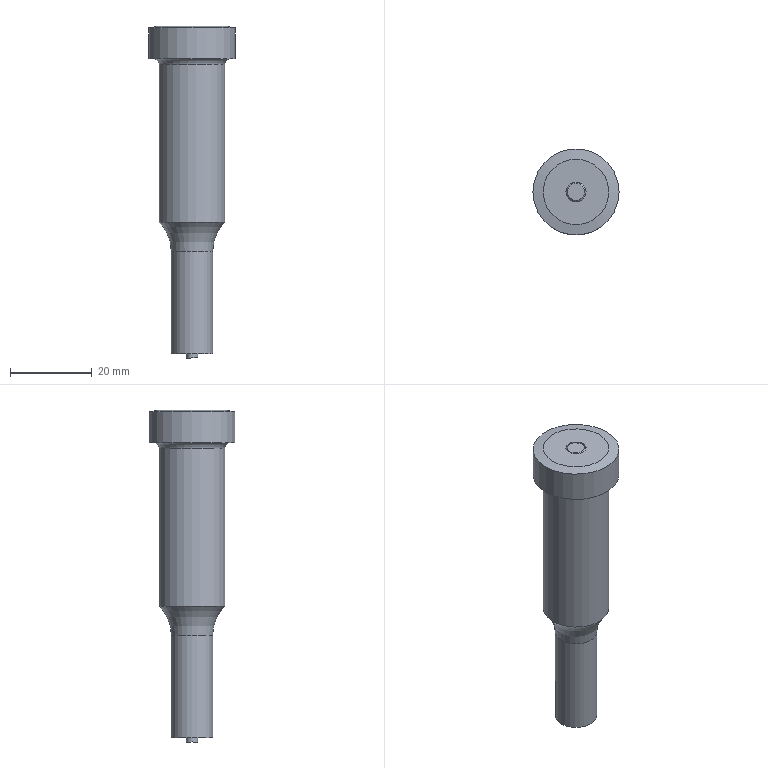Part | STEP file | 1_id3214_x_t | 1 solid | 22 faces | box 21 x 21 x 81 mm | volume 13603 mm3 | cylinder 9 | plane 8 | cone 2 | torus 2 | spline 1 | commonest cylinder face diameters 2.8 x2 4.4 x1 4.401 x1 4.9 x1 4.901 x1 10.1 x1